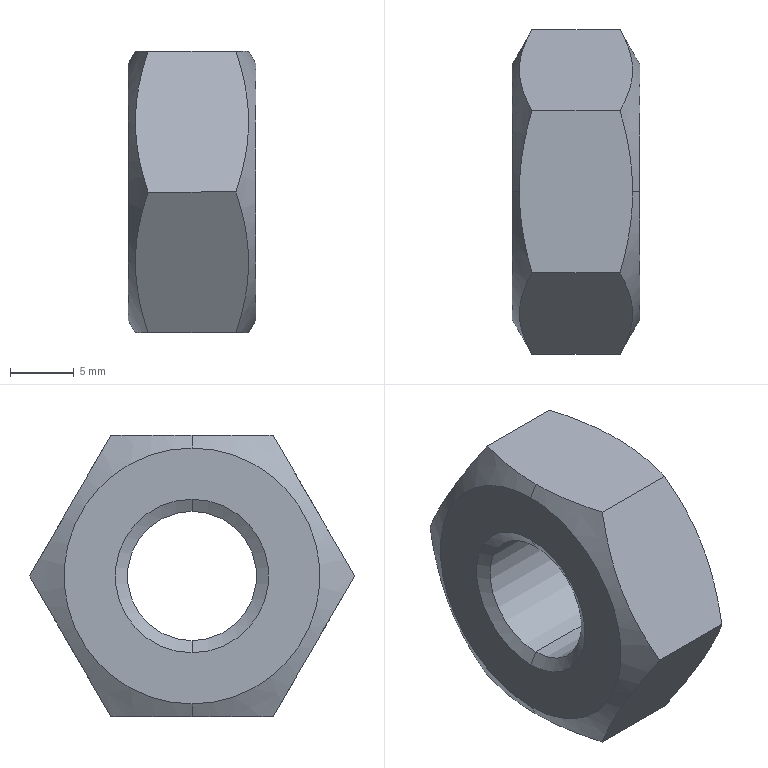Part | STEP file | DIN 6915 M12 | 1 solid | 18 faces | box 10 x 25.403 x 22 mm | volume 3265 mm3 | cone 8 | plane 8 | cylinder 2 | commonest cylinder face diameters 10.106 x2